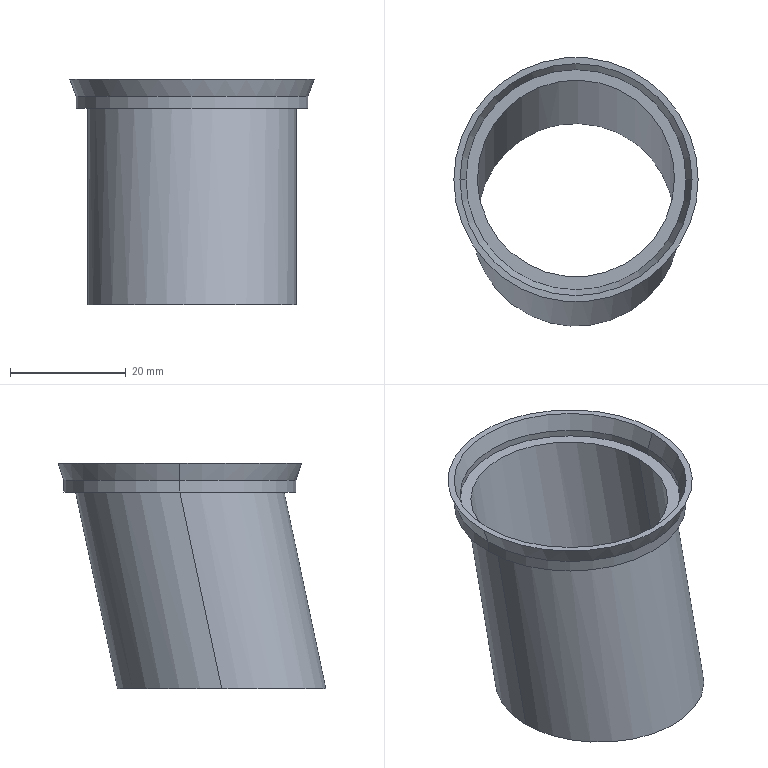Part | SolidWorks | features Extrusion 1, ICE 1, Shell 1, Sweep 1 | 1 solid | 16 faces | box 42.184 x 46.319 x 39 mm | volume 4653 mm3 | cone 4 | cylinder 4 | spline 4 | plane 4 | commonest cylinder face diameters 38 x2 40 x2
STEP:
#1=CARTESIAN_POINT('',(-19.,0.,0.1763));
#2=VERTEX_POINT('',#1);
#3=CARTESIAN_POINT('',(19.,0.,0.1763));
#4=VERTEX_POINT('',#3);
#5=CARTESIAN_POINT('',(0.,0.,0.1763));
#6=DIRECTION('',(0.,0.,1.));
#7=DIRECTION('',(1.,0.,0.));
#8=AXIS2_PLACEMENT_3D('',#5,#6,#7);
#9=CIRCLE('',#8,19.);
#10=EDGE_CURVE('',#2,#4,#9,.T.);
#11=ORIENTED_EDGE('',*,*,#10,.F.);
#12=CARTESIAN_POINT('',(-20.028,0.,3.));
#13=VERTEX_POINT('',#12);
#14=CARTESIAN_POINT('',(-19.06,0.,0.342));
#15=DIRECTION('',(-0.342,0.,0.9397));
#16=VECTOR('',#15,1000.);
#17=LINE('',#14,#16);
#18=EDGE_CURVE('',#2,#13,#17,.T.);
#19=ORIENTED_EDGE('',*,*,#18,.T.);
#20=CARTESIAN_POINT('',(20.028,0.,3.));
#21=VERTEX_POINT('',#20);
#22=CARTESIAN_POINT('',(0.,0.,3.));
#23=DIRECTION('',(0.,0.,1.));
#24=DIRECTION('',(1.,0.,0.));
#25=AXIS2_PLACEMENT_3D('',#22,#23,#24);
#26=CIRCLE('',#25,20.028);
#27=EDGE_CURVE('',#13,#21,#26,.T.);
#28=ORIENTED_EDGE('',*,*,#27,.T.);
#29=CARTESIAN_POINT('',(19.06,0.,0.342));
#30=DIRECTION('',(0.342,0.,0.9397));
#31=VECTOR('',#30,1000.);
#32=LINE('',#29,#31);
#33=EDGE_CURVE('',#4,#21,#32,.T.);
#34=ORIENTED_EDGE('',*,*,#33,.F.);
#35=EDGE_LOOP('',(#11,#19,#28,#34));
#36=FACE_OUTER_BOUND('',#35,.T.);
#37=CARTESIAN_POINT('',(0.,0.,0.342));
#38=DIRECTION('',(0.,0.,1.));
#39=DIRECTION('',(1.,0.,0.));
#40=AXIS2_PLACEMENT_3D('',#37,#38,#39);
#41=CONICAL_SURFACE('',#40,19.06,0.3491);
#42=ADVANCED_FACE('',(#36),#41,.F.);
#43=CARTESIAN_POINT('',(-19.,0.,-1.));
#44=VERTEX_POINT('',#43);
#45=CARTESIAN_POINT('',(19.,0.,-1.));
#46=VERTEX_POINT('',#45);
#47=CARTESIAN_POINT('',(0.,0.,-1.));
#48=DIRECTION('',(0.,0.,1.));
#49=DIRECTION('',(1.,0.,0.));
#50=AXIS2_PLACEMENT_3D('',#47,#48,#49);
#51=CIRCLE('',#50,19.);
#52=EDGE_CURVE('',#44,#46,#51,.T.);
#53=ORIENTED_EDGE('',*,*,#52,.F.);
#54=CARTESIAN_POINT('',(-19.,0.,-2.));
#55=DIRECTION('',(0.,0.,1.));
#56=VECTOR('',#55,1000.);
#57=LINE('',#54,#56);
#58=EDGE_CURVE('',#44,#2,#57,.T.);
#59=ORIENTED_EDGE('',*,*,#58,.T.);
#60=ORIENTED_EDGE('',*,*,#10,.T.);
#61=CARTESIAN_POINT('',(19.,0.,-2.));
#62=DIRECTION('',(0.,0.,1.));
#63=VECTOR('',#62,1000.);
#64=LINE('',#61,#63);
#65=EDGE_CURVE('',#46,#4,#64,.T.);
#66=ORIENTED_EDGE('',*,*,#65,.F.);
#67=EDGE_LOOP('',(#53,#59,#60,#66));
#68=FACE_OUTER_BOUND('',#67,.T.);
#69=CARTESIAN_POINT('',(0.,0.,-2.));
#70=DIRECTION('',(0.,0.,1.));
#71=DIRECTION('',(1.,0.,0.));
#72=AXIS2_PLACEMENT_3D('',#69,#70,#71);
#73=CYLINDRICAL_SURFACE('',#72,19.);
#74=ADVANCED_FACE('',(#68),#73,.F.);
#75=CARTESIAN_POINT('',(-17.,-7.227,-36.));
#76=VERTEX_POINT('',#75);
#77=CARTESIAN_POINT('',(17.,-7.227,-36.));
#78=VERTEX_POINT('',#77);
#79=CARTESIAN_POINT('',(-17.,-7.227,-36.));
#80=CARTESIAN_POINT('',(-17.,-6.117,-36.));
#81=CARTESIAN_POINT('',(-16.892,-5.016,-36.));
#82=CARTESIAN_POINT('',(-16.567,-3.377,-36.));
#83=CARTESIAN_POINT('',(-16.43,-2.83,-36.));
#84=CARTESIAN_POINT('',(-16.105,-1.764,-36.));
#85=CARTESIAN_POINT('',(-15.918,-1.242,-36.));
#86=CARTESIAN_POINT('',(-15.282,0.2919,-36.));
#87=CARTESIAN_POINT('',(-14.76,1.271,-36.));
#88=CARTESIAN_POINT('',(-13.512,3.136,-36.));
#89=CARTESIAN_POINT('',(-12.807,3.992,-36.));
#90=CARTESIAN_POINT('',(-11.633,5.166,-36.));
#91=CARTESIAN_POINT('',(-11.222,5.539,-36.));
#92=CARTESIAN_POINT('',(-10.359,6.246,-36.));
#93=CARTESIAN_POINT('',(-9.906,6.581,-36.));
#94=CARTESIAN_POINT('',(-8.518,7.508,-36.));
#95=CARTESIAN_POINT('',(-7.541,8.029,-36.));
#96=CARTESIAN_POINT('',(-6.003,8.667,-36.));
#97=CARTESIAN_POINT('',(-5.475,8.856,-36.));
#98=CARTESIAN_POINT('',(-4.404,9.181,-36.));
#99=CARTESIAN_POINT('',(-3.864,9.316,-36.));
#100=CARTESIAN_POINT('',(-2.234,9.64,-36.));
#101=CARTESIAN_POINT('',(-1.132,9.75,-36.));
#102=CARTESIAN_POINT('',(0.544,9.751,-36.));
#103=CARTESIAN_POINT('',(1.106,9.724,-36.));
#104=CARTESIAN_POINT('',(2.212,9.616,-36.));
#105=CARTESIAN_POINT('',(3.308,9.454,-36.));
#106=CARTESIAN_POINT('',(4.383,9.186,-36.));
#107=CARTESIAN_POINT('',(5.447,8.865,-36.));
#108=CARTESIAN_POINT('',(5.977,8.677,-36.));
#109=CARTESIAN_POINT('',(7.526,8.037,-36.));
#110=CARTESIAN_POINT('',(8.503,7.516,-36.));
#111=CARTESIAN_POINT('',(9.887,6.595,-36.));
#112=CARTESIAN_POINT('',(10.334,6.265,-36.));
#113=CARTESIAN_POINT('',(11.201,5.557,-36.));
#114=CARTESIAN_POINT('',(11.617,5.181,-36.));
#115=CARTESIAN_POINT('',(12.796,4.005,-36.));
#116=CARTESIAN_POINT('',(13.5,3.151,-36.));
#117=CARTESIAN_POINT('',(14.431,1.765,-36.));
#118=CARTESIAN_POINT('',(14.721,1.283,-36.));
#119=CARTESIAN_POINT('',(15.249,0.2992,-36.));
#120=CARTESIAN_POINT('',(15.486,-0.2022,-36.));
#121=CARTESIAN_POINT('',(16.124,-1.735,-36.));
#122=CARTESIAN_POINT('',(16.449,-2.795,-36.));
#123=CARTESIAN_POINT('',(16.89,-4.994,-36.));
#124=CARTESIAN_POINT('',(17.,-6.107,-36.));
#125=CARTESIAN_POINT('',(17.,-7.227,-36.));
#126=B_SPLINE_CURVE_WITH_KNOTS('',3,(#79,#80,#81,#82,#83,#84,#85,#86,#87,#88,#89,#90,#91,#92,#93,#94,#95,#96,#97,#98,#99,#100,#101,#102,#103,#104,#105,#106,#107,#108,#109,#110,#111,#112,#113,#114,#115,#116,#117,#118,#119,#120,#121,#122,#123,#124,#125),.UNSPECIFIED.,.F.,.F.,(4,2,2,2,2,2,2,2,2,2,2,2,2,1,2,2,2,2,2,2,2,2,2,4),(0.05282,0.05614,0.0578,0.05946,0.06278,0.0661,0.06776,0.06941,0.07273,0.07439,0.07605,0.07937,0.08103,0.08269,0.08435,0.08601,0.08933,0.09099,0.09265,0.09597,0.09763,0.09929,0.1026,0.1059),.UNSPECIFIED.);
#127=EDGE_CURVE('',#76,#78,#126,.T.);
#128=ORIENTED_EDGE('',*,*,#127,.T.);
#129=CARTESIAN_POINT('',(17.,0.2126,-1.));
#130=VERTEX_POINT('',#129);
#131=CARTESIAN_POINT('',(17.,-9.356,-46.017));
#132=DIRECTION('',(0.,0.2079,0.9781));
#133=VECTOR('',#132,1000.);
#134=LINE('',#131,#133);
#135=EDGE_CURVE('',#78,#130,#134,.T.);
#136=ORIENTED_EDGE('',*,*,#135,.T.);
#137=CARTESIAN_POINT('',(-17.,0.2126,-1.));
#138=VERTEX_POINT('',#137);
#139=CARTESIAN_POINT('',(-17.,0.2126,-1.));
#140=CARTESIAN_POINT('',(-17.,1.322,-1.));
#141=CARTESIAN_POINT('',(-16.892,2.423,-1.));
#142=CARTESIAN_POINT('',(-16.566,4.063,-1.));
#143=CARTESIAN_POINT('',(-16.429,4.61,-1.));
#144=CARTESIAN_POINT('',(-16.105,5.676,-1.));
#145=CARTESIAN_POINT('',(-15.918,6.198,-1.));
#146=CARTESIAN_POINT('',(-15.494,7.22,-1.));
#147=CARTESIAN_POINT('',(-15.258,7.72,-1.));
#148=CARTESIAN_POINT('',(-14.734,8.699,-1.));
#149=CARTESIAN_POINT('',(-14.447,9.178,-1.));
#150=CARTESIAN_POINT('',(-13.512,10.576,-1.));
#151=CARTESIAN_POINT('',(-12.808,11.431,-1.));
#152=CARTESIAN_POINT('',(-11.633,12.605,-1.));
#153=CARTESIAN_POINT('',(-11.222,12.978,-1.));
#154=CARTESIAN_POINT('',(-10.358,13.686,-1.));
#155=CARTESIAN_POINT('',(-9.906,14.021,-1.));
#156=CARTESIAN_POINT('',(-8.518,14.947,-1.));
#157=CARTESIAN_POINT('',(-7.542,15.468,-1.));
#158=CARTESIAN_POINT('',(-6.003,16.106,-1.));
#159=CARTESIAN_POINT('',(-5.474,16.296,-1.));
#160=CARTESIAN_POINT('',(-4.404,16.62,-1.));
#161=CARTESIAN_POINT('',(-3.865,16.755,-1.));
#162=CARTESIAN_POINT('',(-2.235,17.079,-1.));
#163=CARTESIAN_POINT('',(-1.133,17.189,-1.));
#164=CARTESIAN_POINT('',(0.5447,17.191,-1.));
#165=CARTESIAN_POINT('',(1.106,17.163,-1.));
#166=CARTESIAN_POINT('',(2.211,17.055,-1.));
#167=CARTESIAN_POINT('',(3.307,16.893,-1.));
#168=CARTESIAN_POINT('',(4.382,16.626,-1.));
#169=CARTESIAN_POINT('',(5.447,16.305,-1.));
#170=CARTESIAN_POINT('',(5.977,16.116,-1.));
#171=CARTESIAN_POINT('',(7.525,15.477,-1.));
#172=CARTESIAN_POINT('',(8.502,14.956,-1.));
#173=CARTESIAN_POINT('',(9.886,14.035,-1.));
#174=CARTESIAN_POINT('',(10.334,13.705,-1.));
#175=CARTESIAN_POINT('',(11.201,12.996,-1.));
#176=CARTESIAN_POINT('',(11.616,12.621,-1.));
#177=CARTESIAN_POINT('',(12.796,11.445,-1.));
#178=CARTESIAN_POINT('',(13.499,10.591,-1.));
#179=CARTESIAN_POINT('',(14.431,9.205,-1.));
#180=CARTESIAN_POINT('',(14.721,8.722,-1.));
#181=CARTESIAN_POINT('',(15.248,7.739,-1.));
#182=CARTESIAN_POINT('',(15.486,7.238,-1.));
#183=CARTESIAN_POINT('',(16.124,5.705,-1.));
#184=CARTESIAN_POINT('',(16.449,4.645,-1.));
#185=CARTESIAN_POINT('',(16.89,2.444,-1.));
#186=CARTESIAN_POINT('',(17.,1.334,-1.));
#187=CARTESIAN_POINT('',(17.,0.2126,-1.));
#188=B_SPLINE_CURVE_WITH_KNOTS('',3,(#139,#140,#141,#142,#143,#144,#145,#146,#147,#148,#149,#150,#151,#152,#153,#154,#155,#156,#157,#158,#159,#160,#161,#162,#163,#164,#165,#166,#167,#168,#169,#170,#171,#172,#173,#174,#175,#176,#177,#178,#179,#180,#181,#182,#183,#184,#185,#186,#187),.UNSPECIFIED.,.F.,.F.,(4,2,2,2,2,2,2,2,2,2,2,2,2,2,1,2,2,2,2,2,2,2,2,2,4),(0.05292,0.05623,0.05789,0.05955,0.06121,0.06287,0.06619,0.06785,0.06951,0.07283,0.07449,0.07615,0.07947,0.08113,0.08279,0.08445,0.08611,0.08943,0.09108,0.09274,0.09606,0.09772,0.09938,0.1027,0.106),.UNSPECIFIED.);
#189=EDGE_CURVE('',#138,#130,#188,.T.);
#190=ORIENTED_EDGE('',*,*,#189,.F.);
#191=CARTESIAN_POINT('',(-17.,-9.356,-46.017));
#192=DIRECTION('',(0.,0.2079,0.9781));
#193=VECTOR('',#192,1000.);
#194=LINE('',#191,#193);
#195=EDGE_CURVE('',#76,#138,#194,.T.);
#196=ORIENTED_EDGE('',*,*,#195,.F.);
#197=EDGE_LOOP('',(#128,#136,#190,#196));
#198=FACE_OUTER_BOUND('',#197,.T.);
#199=CARTESIAN_POINT('',(-17.,-7.316,-36.42));
#200=CARTESIAN_POINT('',(-17.,0.2575,-0.7887));
#201=CARTESIAN_POINT('',(-17.,-6.203,-36.406));
#202=CARTESIAN_POINT('',(-17.,1.37,-0.7748));
#203=CARTESIAN_POINT('',(-16.891,-5.091,-36.392));
#204=CARTESIAN_POINT('',(-16.891,2.483,-0.7609));
#205=CARTESIAN_POINT('',(-16.458,-2.908,-36.365));
#206=CARTESIAN_POINT('',(-16.458,4.666,-0.7337));
#207=CARTESIAN_POINT('',(-16.134,-1.838,-36.351));
#208=CARTESIAN_POINT('',(-16.134,5.736,-0.7204));
#209=CARTESIAN_POINT('',(-15.284,0.2193,-36.326));
#210=CARTESIAN_POINT('',(-15.284,7.793,-0.6949));
#211=CARTESIAN_POINT('',(-14.758,1.206,-36.314));
#212=CARTESIAN_POINT('',(-14.758,8.78,-0.6828));
#213=CARTESIAN_POINT('',(-13.523,3.059,-36.291));
#214=CARTESIAN_POINT('',(-13.523,10.632,-0.6601));
#215=CARTESIAN_POINT('',(-12.815,3.924,-36.281));
#216=CARTESIAN_POINT('',(-12.815,11.498,-0.6496));
#217=CARTESIAN_POINT('',(-11.242,5.501,-36.262));
#218=CARTESIAN_POINT('',(-11.242,13.074,-0.6306));
#219=CARTESIAN_POINT('',(-10.378,6.212,-36.253));
#220=CARTESIAN_POINT('',(-10.378,13.785,-0.6221));
#221=CARTESIAN_POINT('',(-8.528,7.451,-36.238));
#222=CARTESIAN_POINT('',(-8.528,15.025,-0.6073));
#223=CARTESIAN_POINT('',(-7.541,7.98,-36.232));
#224=CARTESIAN_POINT('',(-7.541,15.554,-0.6011));
#225=CARTESIAN_POINT('',(-5.484,8.834,-36.222));
#226=CARTESIAN_POINT('',(-5.484,16.408,-0.591));
#227=CARTESIAN_POINT('',(-4.413,9.16,-36.218));
#228=CARTESIAN_POINT('',(-4.413,16.734,-0.5872));
#229=CARTESIAN_POINT('',(-2.228,9.596,-36.213));
#230=CARTESIAN_POINT('',(-2.228,17.169,-0.5821));
#231=CARTESIAN_POINT('',(-1.114,9.706,-36.212));
#232=CARTESIAN_POINT('',(-1.114,17.279,-0.5808));
#233=CARTESIAN_POINT('',(1.114,9.706,-36.212));
#234=CARTESIAN_POINT('',(1.114,17.279,-0.5808));
#235=CARTESIAN_POINT('',(2.228,9.596,-36.213));
#236=CARTESIAN_POINT('',(2.228,17.169,-0.5821));
#237=CARTESIAN_POINT('',(4.413,9.16,-36.218));
#238=CARTESIAN_POINT('',(4.413,16.734,-0.5872));
#239=CARTESIAN_POINT('',(5.484,8.834,-36.222));
#240=CARTESIAN_POINT('',(5.484,16.408,-0.591));
#241=CARTESIAN_POINT('',(7.541,7.98,-36.232));
#242=CARTESIAN_POINT('',(7.541,15.554,-0.6011));
#243=CARTESIAN_POINT('',(8.528,7.451,-36.238));
#244=CARTESIAN_POINT('',(8.528,15.025,-0.6073));
#245=CARTESIAN_POINT('',(10.378,6.212,-36.253));
#246=CARTESIAN_POINT('',(10.378,13.785,-0.6221));
#247=CARTESIAN_POINT('',(11.242,5.501,-36.262));
#248=CARTESIAN_POINT('',(11.242,13.074,-0.6306));
#249=CARTESIAN_POINT('',(12.815,3.924,-36.281));
#250=CARTESIAN_POINT('',(12.815,11.498,-0.6496));
#251=CARTESIAN_POINT('',(13.523,3.059,-36.291));
#252=CARTESIAN_POINT('',(13.523,10.632,-0.6601));
#253=CARTESIAN_POINT('',(14.758,1.206,-36.314));
#254=CARTESIAN_POINT('',(14.758,8.78,-0.6828));
#255=CARTESIAN_POINT('',(15.284,0.2193,-36.326));
#256=CARTESIAN_POINT('',(15.284,7.793,-0.6949));
#257=CARTESIAN_POINT('',(16.134,-1.838,-36.351));
#258=CARTESIAN_POINT('',(16.134,5.736,-0.7204));
#259=CARTESIAN_POINT('',(16.458,-2.908,-36.365));
#260=CARTESIAN_POINT('',(16.458,4.666,-0.7337));
#261=CARTESIAN_POINT('',(16.891,-5.091,-36.392));
#262=CARTESIAN_POINT('',(16.891,2.483,-0.7609));
#263=CARTESIAN_POINT('',(17.,-6.203,-36.406));
#264=CARTESIAN_POINT('',(17.,1.37,-0.7748));
#265=CARTESIAN_POINT('',(17.,-7.316,-36.42));
#266=CARTESIAN_POINT('',(17.,0.2575,-0.7887));
#267=B_SPLINE_SURFACE_WITH_KNOTS('',3,1,((#199,#200),(#201,#202),(#203,#204),(#205,#206),(#207,#208),(#209,#210),(#211,#212),(#213,#214),(#215,#216),(#217,#218),(#219,#220),(#221,#222),(#223,#224),(#225,#226),(#227,#228),(#229,#230),(#231,#232),(#233,#234),(#235,#236),(#237,#238),(#239,#240),(#241,#242),(#243,#244),(#245,#246),(#247,#248),(#249,#250),(#251,#252),(#253,#254),(#255,#256),(#257,#258),(#259,#260),(#261,#262),(#263,#264),(#265,#266)),.UNSPECIFIED.,.F.,.F.,.F.,(4,2,2,2,2,2,2,2,2,2,2,2,2,2,2,2,4),(2,2),(0.,0.0625,0.125,0.1875,0.25,0.3125,0.375,0.4375,0.5,0.5625,0.625,0.6875,0.75,0.8125,0.875,0.9375,1.),(0.,1.),.UNSPECIFIED.);
#268=ADVANCED_FACE('',(#198),#267,.T.);
#269=CARTESIAN_POINT('',(20.,0.,0.));
#270=VERTEX_POINT('',#269);
#271=CARTESIAN_POINT('',(-20.,0.,0.));
#272=VERTEX_POINT('',#271);
#273=CARTESIAN_POINT('',(0.,0.,0.));
#274=DIRECTION('',(0.,0.,1.));
#275=DIRECTION('',(1.,0.,0.));
#276=AXIS2_PLACEMENT_3D('',#273,#274,#275);
#277=CIRCLE('',#276,20.);
#278=EDGE_CURVE('',#270,#272,#277,.T.);
#279=ORIENTED_EDGE('',*,*,#278,.T.);
#280=CARTESIAN_POINT('',(-21.092,0.,3.));
#281=VERTEX_POINT('',#280);
#282=CARTESIAN_POINT('',(-20.,0.,0.));
#283=DIRECTION('',(-0.342,0.,0.9397));
#284=VECTOR('',#283,1000.);
#285=LINE('',#282,#284);
#286=EDGE_CURVE('',#272,#281,#285,.T.);
#287=ORIENTED_EDGE('',*,*,#286,.T.);
#288=CARTESIAN_POINT('',(21.092,0.,3.));
#289=VERTEX_POINT('',#288);
#290=CARTESIAN_POINT('',(0.,0.,3.));
#291=DIRECTION('',(0.,0.,1.));
#292=DIRECTION('',(1.,0.,0.));
#293=AXIS2_PLACEMENT_3D('',#290,#291,#292);
#294=CIRCLE('',#293,21.092);
#295=EDGE_CURVE('',#289,#281,#294,.T.);
#296=ORIENTED_EDGE('',*,*,#295,.F.);
#297=CARTESIAN_POINT('',(20.,0.,0.));
#298=DIRECTION('',(0.342,0.,0.9397));
#299=VECTOR('',#298,1000.);
#300=LINE('',#297,#299);
#301=EDGE_CURVE('',#270,#289,#300,.T.);
#302=ORIENTED_EDGE('',*,*,#301,.F.);
#303=EDGE_LOOP('',(#279,#287,#296,#302));
#304=FACE_OUTER_BOUND('',#303,.T.);
#305=CARTESIAN_POINT('',(0.,0.,0.));
#306=DIRECTION('',(0.,0.,1.));
#307=DIRECTION('',(1.,0.,0.));
#308=AXIS2_PLACEMENT_3D('',#305,#306,#307);
#309=CONICAL_SURFACE('',#308,20.,0.3491);
#310=ADVANCED_FACE('',(#304),#309,.T.);
#311=CARTESIAN_POINT('',(20.,0.,-2.));
#312=VERTEX_POINT('',#311);
#313=CARTESIAN_POINT('',(-20.,0.,-2.));
#314=VERTEX_POINT('',#313);
#315=CARTESIAN_POINT('',(0.,0.,-2.));
#316=DIRECTION('',(0.,0.,1.));
#317=DIRECTION('',(1.,0.,0.));
#318=AXIS2_PLACEMENT_3D('',#315,#316,#317);
#319=CIRCLE('',#318,20.);
#320=EDGE_CURVE('',#312,#314,#319,.T.);
#321=ORIENTED_EDGE('',*,*,#320,.T.);
#322=CARTESIAN_POINT('',(-20.,0.,-2.));
#323=DIRECTION('',(0.,0.,1.));
#324=VECTOR('',#323,1000.);
#325=LINE('',#322,#324);
#326=EDGE_CURVE('',#314,#272,#325,.T.);
#327=ORIENTED_EDGE('',*,*,#326,.T.);
#328=ORIENTED_EDGE('',*,*,#278,.F.);
#329=CARTESIAN_POINT('',(20.,0.,-2.));
#330=DIRECTION('',(0.,0.,1.));
#331=VECTOR('',#330,1000.);
#332=LINE('',#329,#331);
#333=EDGE_CURVE('',#312,#270,#332,.T.);
#334=ORIENTED_EDGE('',*,*,#333,.F.);
#335=EDGE_LOOP('',(#321,#327,#328,#334));
#336=FACE_OUTER_BOUND('',#335,.T.);
#337=CARTESIAN_POINT('',(0.,0.,-2.));
#338=DIRECTION('',(0.,0.,1.));
#339=DIRECTION('',(1.,0.,0.));
#340=AXIS2_PLACEMENT_3D('',#337,#338,#339);
#341=CYLINDRICAL_SURFACE('',#340,20.);
#342=ADVANCED_FACE('',(#336),#341,.T.);
#343=CARTESIAN_POINT('',(18.,-7.227,-36.));
#344=VERTEX_POINT('',#343);
#345=CARTESIAN_POINT('',(-18.,-7.227,-36.));
#346=VERTEX_POINT('',#345);
#347=CARTESIAN_POINT('',(18.,-7.227,-36.));
#348=CARTESIAN_POINT('',(18.,-8.406,-36.));
#349=CARTESIAN_POINT('',(17.884,-9.582,-36.));
#350=CARTESIAN_POINT('',(17.539,-11.317,-36.));
#351=CARTESIAN_POINT('',(17.396,-11.888,-36.));
#352=CARTESIAN_POINT('',(17.054,-13.015,-36.));
#353=CARTESIAN_POINT('',(16.855,-13.572,-36.));
#354=CARTESIAN_POINT('',(16.404,-14.659,-36.));
#355=CARTESIAN_POINT('',(16.153,-15.191,-36.));
#356=CARTESIAN_POINT('',(15.597,-16.231,-36.));
#357=CARTESIAN_POINT('',(15.294,-16.738,-36.));
#358=CARTESIAN_POINT('',(14.313,-18.205,-36.));
#359=CARTESIAN_POINT('',(13.561,-19.122,-36.));
#360=CARTESIAN_POINT('',(12.313,-20.37,-36.));
#361=CARTESIAN_POINT('',(11.875,-20.767,-36.));
#362=CARTESIAN_POINT('',(10.964,-21.514,-36.));
#363=CARTESIAN_POINT('',(10.492,-21.865,-36.));
#364=CARTESIAN_POINT('',(9.512,-22.519,-36.));
#365=CARTESIAN_POINT('',(9.005,-22.823,-36.));
#366=CARTESIAN_POINT('',(7.968,-23.378,-36.));
#367=CARTESIAN_POINT('',(7.436,-23.63,-36.));
#368=CARTESIAN_POINT('',(6.345,-24.082,-36.));
#369=CARTESIAN_POINT('',(5.79,-24.28,-36.));
#370=CARTESIAN_POINT('',(4.665,-24.622,-36.));
#371=CARTESIAN_POINT('',(4.091,-24.766,-36.));
#372=CARTESIAN_POINT('',(2.936,-24.996,-36.));
#373=CARTESIAN_POINT('',(2.354,-25.082,-36.));
#374=CARTESIAN_POINT('',(1.182,-25.198,-36.));
#375=CARTESIAN_POINT('',(0.5909,-25.227,-36.));
#376=CARTESIAN_POINT('',(-1.175,-25.227,-36.));
#377=CARTESIAN_POINT('',(-2.354,-25.111,-36.));
#378=CARTESIAN_POINT('',(-4.085,-24.767,-36.));
#379=CARTESIAN_POINT('',(-4.658,-24.624,-36.));
#380=CARTESIAN_POINT('',(-5.786,-24.282,-36.));
#381=CARTESIAN_POINT('',(-6.34,-24.084,-36.));
#382=CARTESIAN_POINT('',(-7.428,-23.633,-36.));
#383=CARTESIAN_POINT('',(-7.963,-23.38,-36.));
#384=CARTESIAN_POINT('',(-9.001,-22.826,-36.));
#385=CARTESIAN_POINT('',(-9.506,-22.523,-36.));
#386=CARTESIAN_POINT('',(-10.977,-21.541,-36.));
#387=CARTESIAN_POINT('',(-11.891,-20.792,-36.));
#388=CARTESIAN_POINT('',(-13.142,-19.541,-36.));
#389=CARTESIAN_POINT('',(-13.537,-19.105,-36.));
#390=CARTESIAN_POINT('',(-14.284,-18.195,-36.));
#391=CARTESIAN_POINT('',(-14.637,-17.72,-36.));
#392=CARTESIAN_POINT('',(-15.291,-16.741,-36.));
#393=CARTESIAN_POINT('',(-15.594,-16.237,-36.));
#394=CARTESIAN_POINT('',(-16.15,-15.198,-36.));
#395=CARTESIAN_POINT('',(-16.403,-14.664,-36.));
#396=CARTESIAN_POINT('',(-17.078,-13.033,-36.));
#397=CARTESIAN_POINT('',(-17.423,-11.899,-36.));
#398=CARTESIAN_POINT('',(-17.883,-9.589,-36.));
#399=CARTESIAN_POINT('',(-18.,-8.408,-36.));
#400=CARTESIAN_POINT('',(-18.,-7.227,-36.));
#401=B_SPLINE_CURVE_WITH_KNOTS('',3,(#347,#348,#349,#350,#351,#352,#353,#354,#355,#356,#357,#358,#359,#360,#361,#362,#363,#364,#365,#366,#367,#368,#369,#370,#371,#372,#373,#374,#375,#376,#377,#378,#379,#380,#381,#382,#383,#384,#385,#386,#387,#388,#389,#390,#391,#392,#393,#394,#395,#396,#397,#398,#399,#400),.UNSPECIFIED.,.F.,.F.,(4,2,2,2,2,2,2,2,2,2,2,2,2,2,2,2,2,2,2,2,2,2,2,2,2,2,4),(0.05648,0.06001,0.06178,0.06354,0.06531,0.06707,0.0706,0.07237,0.07413,0.0759,0.07766,0.07943,0.08119,0.08296,0.08472,0.08825,0.09002,0.09178,0.09355,0.09531,0.09884,0.1006,0.1024,0.1041,0.1059,0.1094,0.113),.UNSPECIFIED.);
#402=EDGE_CURVE('',#344,#346,#401,.T.);
#403=ORIENTED_EDGE('',*,*,#402,.F.);
#404=CARTESIAN_POINT('',(18.,0.,-2.));
#405=VERTEX_POINT('',#404);
#406=CARTESIAN_POINT('',(18.,-9.356,-46.017));
#407=DIRECTION('',(0.,0.2079,0.9781));
#408=VECTOR('',#407,1000.);
#409=LINE('',#406,#408);
#410=EDGE_CURVE('',#344,#405,#409,.T.);
#411=ORIENTED_EDGE('',*,*,#410,.T.);
#412=CARTESIAN_POINT('',(-18.,0.,-2.));
#413=VERTEX_POINT('',#412);
#414=CARTESIAN_POINT('',(0.,0.,-2.));
#415=DIRECTION('',(0.,0.,-1.));
#416=DIRECTION('',(-1.,0.,0.));
#417=AXIS2_PLACEMENT_3D('',#414,#415,#416);
#418=CIRCLE('',#417,18.);
#419=EDGE_CURVE('',#405,#413,#418,.T.);
#420=ORIENTED_EDGE('',*,*,#419,.T.);
#421=CARTESIAN_POINT('',(-18.,-9.356,-46.017));
#422=DIRECTION('',(0.,0.2079,0.9781));
#423=VECTOR('',#422,1000.);
#424=LINE('',#421,#423);
#425=EDGE_CURVE('',#346,#413,#424,.T.);
#426=ORIENTED_EDGE('',*,*,#425,.F.);
#427=EDGE_LOOP('',(#403,#411,#420,#426));
#428=FACE_OUTER_BOUND('',#427,.T.);
#429=CARTESIAN_POINT('',(18.,-7.227,-36.));
#430=CARTESIAN_POINT('',(18.,0.,-2.));
#431=CARTESIAN_POINT('',(18.,-43.227,-36.));
#432=CARTESIAN_POINT('',(18.,-36.,-2.));
#433=CARTESIAN_POINT('',(-18.,-43.227,-36.));
#434=CARTESIAN_POINT('',(-18.,-36.,-2.));
#435=CARTESIAN_POINT('',(-18.,-7.227,-36.));
#436=CARTESIAN_POINT('',(-18.,0.,-2.));
#437=(BOUNDED_SURFACE()B_SPLINE_SURFACE(3,1,((#429,#430),(#431,#432),(#433,#434),(#435,#436)),.UNSPECIFIED.,.F.,.F.,.F.)B_SPLINE_SURFACE_WITH_KNOTS((4,4),(2,2),(0.,1.),(0.,1.),.UNSPECIFIED.)GEOMETRIC_REPRESENTATION_ITEM()RATIONAL_B_SPLINE_SURFACE(((1.,1.),(0.3333,0.3333),(0.3333,0.3333),(1.,1.)))REPRESENTATION_ITEM('')SURFACE());
#438=ADVANCED_FACE('',(#428),#437,.F.);
#439=ORIENTED_EDGE('',*,*,#410,.F.);
#440=CARTESIAN_POINT('',(-18.,-7.227,-36.));
#441=CARTESIAN_POINT('',(-18.,-6.637,-36.));
#442=CARTESIAN_POINT('',(-17.971,-6.049,-36.));
#443=CARTESIAN_POINT('',(-17.856,-4.877,-36.));
#444=CARTESIAN_POINT('',(-17.769,-4.293,-36.));
#445=CARTESIAN_POINT('',(-17.539,-3.137,-36.));
#446=CARTESIAN_POINT('',(-17.396,-2.566,-36.));
#447=CARTESIAN_POINT('',(-17.054,-1.439,-36.));
#448=CARTESIAN_POINT('',(-16.855,-0.8819,-36.));
#449=CARTESIAN_POINT('',(-16.179,0.7493,-36.));
#450=CARTESIAN_POINT('',(-15.62,1.795,-36.));
#451=CARTESIAN_POINT('',(-14.64,3.263,-36.));
#452=CARTESIAN_POINT('',(-14.288,3.737,-36.));
#453=CARTESIAN_POINT('',(-13.54,4.648,-36.));
#454=CARTESIAN_POINT('',(-13.145,5.084,-36.));
#455=CARTESIAN_POINT('',(-12.312,5.917,-36.));
#456=CARTESIAN_POINT('',(-11.874,6.314,-36.));
#457=CARTESIAN_POINT('',(-10.963,7.061,-36.));
#458=CARTESIAN_POINT('',(-10.491,7.412,-36.));
#459=CARTESIAN_POINT('',(-9.02,8.395,-36.));
#460=CARTESIAN_POINT('',(-7.977,8.952,-36.));
#461=CARTESIAN_POINT('',(-6.343,9.629,-36.));
#462=CARTESIAN_POINT('',(-5.789,9.827,-36.));
#463=CARTESIAN_POINT('',(-4.662,10.169,-36.));
#464=CARTESIAN_POINT('',(-4.088,10.313,-36.));
#465=CARTESIAN_POINT('',(-2.933,10.542,-36.));
#466=CARTESIAN_POINT('',(-2.351,10.629,-36.));
#467=CARTESIAN_POINT('',(-1.178,10.744,-36.));
#468=CARTESIAN_POINT('',(-0.588,10.773,-36.));
#469=CARTESIAN_POINT('',(1.177,10.773,-36.));
#470=CARTESIAN_POINT('',(2.357,10.657,-36.));
#471=CARTESIAN_POINT('',(4.089,10.312,-36.));
#472=CARTESIAN_POINT('',(4.662,10.169,-36.));
#473=CARTESIAN_POINT('',(5.79,9.827,-36.));
#474=CARTESIAN_POINT('',(6.344,9.628,-36.));
#475=CARTESIAN_POINT('',(7.432,9.178,-36.));
#476=CARTESIAN_POINT('',(7.967,8.925,-36.));
#477=CARTESIAN_POINT('',(9.005,8.37,-36.));
#478=CARTESIAN_POINT('',(9.51,8.067,-36.));
#479=CARTESIAN_POINT('',(10.491,7.411,-36.));
#480=CARTESIAN_POINT('',(10.964,7.061,-36.));
#481=CARTESIAN_POINT('',(11.874,6.314,-36.));
#482=CARTESIAN_POINT('',(12.312,5.917,-36.));
#483=CARTESIAN_POINT('',(13.145,5.084,-36.));
#484=CARTESIAN_POINT('',(13.54,4.648,-36.));
#485=CARTESIAN_POINT('',(14.288,3.737,-36.));
#486=CARTESIAN_POINT('',(14.64,3.262,-36.));
#487=CARTESIAN_POINT('',(15.621,1.794,-36.));
#488=CARTESIAN_POINT('',(16.18,0.7483,-36.));
#489=CARTESIAN_POINT('',(16.855,-0.8825,-36.));
#490=CARTESIAN_POINT('',(17.054,-1.439,-36.));
#491=CARTESIAN_POINT('',(17.396,-2.567,-36.));
#492=CARTESIAN_POINT('',(17.539,-3.138,-36.));
#493=CARTESIAN_POINT('',(17.769,-4.293,-36.));
#494=CARTESIAN_POINT('',(17.856,-4.878,-36.));
#495=CARTESIAN_POINT('',(17.971,-6.05,-36.));
#496=CARTESIAN_POINT('',(18.,-6.637,-36.));
#497=CARTESIAN_POINT('',(18.,-7.227,-36.));
#498=B_SPLINE_CURVE_WITH_KNOTS('',3,(#440,#441,#442,#443,#444,#445,#446,#447,#448,#449,#450,#451,#452,#453,#454,#455,#456,#457,#458,#459,#460,#461,#462,#463,#464,#465,#466,#467,#468,#469,#470,#471,#472,#473,#474,#475,#476,#477,#478,#479,#480,#481,#482,#483,#484,#485,#486,#487,#488,#489,#490,#491,#492,#493,#494,#495,#496,#497),.UNSPECIFIED.,.F.,.F.,(4,2,2,2,2,2,2,2,2,2,2,2,2,2,2,2,2,2,2,2,2,2,2,2,2,2,2,2,4),(0.,0.001765,0.00353,0.005295,0.007061,0.01059,0.01236,0.01412,0.01589,0.01765,0.02118,0.02295,0.02471,0.02648,0.02824,0.03177,0.03354,0.0353,0.03707,0.03883,0.0406,0.04236,0.04413,0.04589,0.04942,0.05119,0.05295,0.05472,0.05648),.UNSPECIFIED.);
#499=EDGE_CURVE('',#346,#344,#498,.T.);
#500=ORIENTED_EDGE('',*,*,#499,.F.);
#501=ORIENTED_EDGE('',*,*,#425,.T.);
#502=CARTESIAN_POINT('',(0.,0.,-2.));
#503=DIRECTION('',(0.,0.,-1.));
#504=DIRECTION('',(-1.,0.,0.));
#505=AXIS2_PLACEMENT_3D('',#502,#503,#504);
#506=CIRCLE('',#505,18.);
#507=EDGE_CURVE('',#413,#405,#506,.T.);
#508=ORIENTED_EDGE('',*,*,#507,.T.);
#509=EDGE_LOOP('',(#439,#500,#501,#508));
#510=FACE_OUTER_BOUND('',#509,.T.);
#511=CARTESIAN_POINT('',(-18.,-7.227,-36.));
#512=CARTESIAN_POINT('',(-18.,0.,-2.));
#513=CARTESIAN_POINT('',(-18.,28.773,-36.));
#514=CARTESIAN_POINT('',(-18.,36.,-2.));
#515=CARTESIAN_POINT('',(18.,28.773,-36.));
#516=CARTESIAN_POINT('',(18.,36.,-2.));
#517=CARTESIAN_POINT('',(18.,-7.227,-36.));
#518=CARTESIAN_POINT('',(18.,0.,-2.));
#519=(BOUNDED_SURFACE()B_SPLINE_SURFACE(3,1,((#511,#512),(#513,#514),(#515,#516),(#517,#518)),.UNSPECIFIED.,.F.,.F.,.F.)B_SPLINE_SURFACE_WITH_KNOTS((4,4),(2,2),(0.,1.),(0.,1.),.UNSPECIFIED.)GEOMETRIC_REPRESENTATION_ITEM()RATIONAL_B_SPLINE_SURFACE(((1.,1.),(0.3333,0.3333),(0.3333,0.3333),(1.,1.)))REPRESENTATION_ITEM('')SURFACE());
#520=ADVANCED_FACE('',(#510),#519,.F.);
#521=ORIENTED_EDGE('',*,*,#320,.F.);
#522=CARTESIAN_POINT('',(0.,0.,-2.));
#523=DIRECTION('',(0.,0.,1.));
#524=DIRECTION('',(1.,0.,0.));
#525=AXIS2_PLACEMENT_3D('',#522,#523,#524);
#526=CIRCLE('',#525,20.);
#527=EDGE_CURVE('',#314,#312,#526,.T.);
#528=ORIENTED_EDGE('',*,*,#527,.F.);
#529=EDGE_LOOP('',(#521,#528));
#530=FACE_OUTER_BOUND('',#529,.T.);
#531=ORIENTED_EDGE('',*,*,#507,.F.);
#532=ORIENTED_EDGE('',*,*,#419,.F.);
#533=EDGE_LOOP('',(#531,#532));
#534=FACE_BOUND('',#533,.T.);
#535=CARTESIAN_POINT('',(0.,0.,-2.));
#536=DIRECTION('',(0.,0.,1.));
#537=DIRECTION('',(1.,0.,0.));
#538=AXIS2_PLACEMENT_3D('',#535,#536,#537);
#539=PLANE('',#538);
#540=ADVANCED_FACE('',(#530,#534),#539,.F.);
#541=ORIENTED_EDGE('',*,*,#326,.F.);
#542=ORIENTED_EDGE('',*,*,#527,.T.);
#543=ORIENTED_EDGE('',*,*,#333,.T.);
#544=CARTESIAN_POINT('',(0.,0.,0.));
#545=DIRECTION('',(0.,0.,1.));
#546=DIRECTION('',(1.,0.,0.));
#547=AXIS2_PLACEMENT_3D('',#544,#545,#546);
#548=CIRCLE('',#547,20.);
#549=EDGE_CURVE('',#272,#270,#548,.T.);
#550=ORIENTED_EDGE('',*,*,#549,.F.);
#551=EDGE_LOOP('',(#541,#542,#543,#550));
#552=FACE_OUTER_BOUND('',#551,.T.);
#553=CARTESIAN_POINT('',(0.,0.,-2.));
#554=DIRECTION('',(0.,0.,1.));
#555=DIRECTION('',(1.,0.,0.));
#556=AXIS2_PLACEMENT_3D('',#553,#554,#555);
#557=CYLINDRICAL_SURFACE('',#556,20.);
#558=ADVANCED_FACE('',(#552),#557,.T.);
#559=ORIENTED_EDGE('',*,*,#286,.F.);
#560=ORIENTED_EDGE('',*,*,#549,.T.);
#561=ORIENTED_EDGE('',*,*,#301,.T.);
#562=CARTESIAN_POINT('',(0.,0.,3.));
#563=DIRECTION('',(0.,0.,1.));
#564=DIRECTION('',(1.,0.,0.));
#565=AXIS2_PLACEMENT_3D('',#562,#563,#564);
#566=CIRCLE('',#565,21.092);
#567=EDGE_CURVE('',#281,#289,#566,.T.);
#568=ORIENTED_EDGE('',*,*,#567,.F.);
#569=EDGE_LOOP('',(#559,#560,#561,#568));
#570=FACE_OUTER_BOUND('',#569,.T.);
#571=CARTESIAN_POINT('',(0.,0.,0.));
#572=DIRECTION('',(0.,0.,1.));
#573=DIRECTION('',(1.,0.,0.));
#574=AXIS2_PLACEMENT_3D('',#571,#572,#573);
#575=CONICAL_SURFACE('',#574,20.,0.3491);
#576=ADVANCED_FACE('',(#570),#575,.T.);
#577=CARTESIAN_POINT('',(0.,0.,3.));
#578=DIRECTION('',(0.,0.,1.));
#579=DIRECTION('',(1.,0.,0.));
#580=AXIS2_PLACEMENT_3D('',#577,#578,#579);
#581=CIRCLE('',#580,20.028);
#582=EDGE_CURVE('',#21,#13,#581,.T.);
#583=ORIENTED_EDGE('',*,*,#582,.F.);
#584=ORIENTED_EDGE('',*,*,#27,.F.);
#585=EDGE_LOOP('',(#583,#584));
#586=FACE_BOUND('',#585,.T.);
#587=ORIENTED_EDGE('',*,*,#295,.T.);
#588=ORIENTED_EDGE('',*,*,#567,.T.);
#589=EDGE_LOOP('',(#587,#588));
#590=FACE_OUTER_BOUND('',#589,.T.);
#591=CARTESIAN_POINT('',(0.,0.,3.));
#592=DIRECTION('',(0.,0.,1.));
#593=DIRECTION('',(1.,0.,0.));
#594=AXIS2_PLACEMENT_3D('',#591,#592,#593);
#595=PLANE('',#594);
#596=ADVANCED_FACE('',(#586,#590),#595,.T.);
#597=ORIENTED_EDGE('',*,*,#127,.F.);
#598=CARTESIAN_POINT('',(17.,-7.227,-36.));
#599=CARTESIAN_POINT('',(17.,-7.787,-36.));
#600=CARTESIAN_POINT('',(16.972,-8.347,-36.));
#601=CARTESIAN_POINT('',(16.863,-9.452,-36.));
#602=CARTESIAN_POINT('',(16.699,-10.547,-36.));
#603=CARTESIAN_POINT('',(16.43,-11.623,-36.));
#604=CARTESIAN_POINT('',(16.106,-12.688,-36.));
#605=CARTESIAN_POINT('',(15.916,-13.218,-36.));
#606=CARTESIAN_POINT('',(15.274,-14.764,-36.));
#607=CARTESIAN_POINT('',(14.751,-15.739,-36.));
#608=CARTESIAN_POINT('',(13.825,-17.122,-36.));
#609=CARTESIAN_POINT('',(13.494,-17.569,-36.));
#610=CARTESIAN_POINT('',(12.781,-18.435,-36.));
#611=CARTESIAN_POINT('',(12.406,-18.848,-36.));
#612=CARTESIAN_POINT('',(11.227,-20.023,-36.));
#613=CARTESIAN_POINT('',(10.371,-20.725,-36.));
#614=CARTESIAN_POINT('',(8.98,-21.653,-36.));
#615=CARTESIAN_POINT('',(8.497,-21.942,-36.));
#616=CARTESIAN_POINT('',(7.513,-22.467,-36.));
#617=CARTESIAN_POINT('',(7.012,-22.703,-36.));
#618=CARTESIAN_POINT('',(5.989,-23.126,-36.));
#619=CARTESIAN_POINT('',(5.468,-23.312,-36.));
#620=CARTESIAN_POINT('',(4.406,-23.634,-36.));
#621=CARTESIAN_POINT('',(3.863,-23.77,-36.));
#622=CARTESIAN_POINT('',(2.214,-24.097,-36.));
#623=CARTESIAN_POINT('',(1.111,-24.204,-36.));
#624=CARTESIAN_POINT('',(-0.55,-24.205,-36.));
#625=CARTESIAN_POINT('',(-1.105,-24.178,-36.));
#626=CARTESIAN_POINT('',(-2.216,-24.069,-36.));
#627=CARTESIAN_POINT('',(-2.773,-23.986,-36.));
#628=CARTESIAN_POINT('',(-4.409,-23.661,-36.));
#629=CARTESIAN_POINT('',(-5.468,-23.34,-36.));
#630=CARTESIAN_POINT('',(-7.009,-22.704,-36.));
#631=CARTESIAN_POINT('',(-7.517,-22.465,-36.));
#632=CARTESIAN_POINT('',(-8.504,-21.938,-36.));
#633=CARTESIAN_POINT('',(-8.981,-21.653,-36.));
#634=CARTESIAN_POINT('',(-10.363,-20.731,-36.));
#635=CARTESIAN_POINT('',(-11.221,-20.03,-36.));
#636=CARTESIAN_POINT('',(-12.408,-18.845,-36.));
#637=CARTESIAN_POINT('',(-12.786,-18.429,-36.));
#638=CARTESIAN_POINT('',(-13.492,-17.571,-36.));
#639=CARTESIAN_POINT('',(-14.152,-16.682,-36.));
#640=CARTESIAN_POINT('',(-14.723,-15.732,-36.));
#641=CARTESIAN_POINT('',(-15.249,-14.752,-36.));
#642=CARTESIAN_POINT('',(-15.49,-14.244,-36.));
#643=CARTESIAN_POINT('',(-16.132,-12.696,-36.));
#644=CARTESIAN_POINT('',(-16.454,-11.637,-36.));
#645=CARTESIAN_POINT('',(-16.78,-10.006,-36.));
#646=CARTESIAN_POINT('',(-16.862,-9.456,-36.));
#647=CARTESIAN_POINT('',(-16.973,-8.341,-36.));
#648=CARTESIAN_POINT('',(-17.,-7.782,-36.));
#649=CARTESIAN_POINT('',(-17.,-7.227,-36.));
#650=B_SPLINE_CURVE_WITH_KNOTS('',3,(#598,#599,#600,#601,#602,#603,#604,#605,#606,#607,#608,#609,#610,#611,#612,#613,#614,#615,#616,#617,#618,#619,#620,#621,#622,#623,#624,#625,#626,#627,#628,#629,#630,#631,#632,#633,#634,#635,#636,#637,#638,#639,#640,#641,#642,#643,#644,#645,#646,#647,#648,#649),.UNSPECIFIED.,.F.,.F.,(4,2,1,2,2,2,2,2,2,2,2,2,2,2,2,2,2,2,2,2,2,1,2,2,2,2,4),(0.1059,0.1076,0.1092,0.1109,0.1126,0.1159,0.1175,0.1192,0.1225,0.1242,0.1258,0.1275,0.1292,0.1325,0.1341,0.1358,0.1391,0.1408,0.1424,0.1458,0.1474,0.1491,0.1507,0.1524,0.1557,0.1574,0.159),.UNSPECIFIED.);
#651=EDGE_CURVE('',#78,#76,#650,.T.);
#652=ORIENTED_EDGE('',*,*,#651,.F.);
#653=EDGE_LOOP('',(#597,#652));
#654=FACE_BOUND('',#653,.T.);
#655=ORIENTED_EDGE('',*,*,#499,.T.);
#656=ORIENTED_EDGE('',*,*,#402,.T.);
#657=EDGE_LOOP('',(#655,#656));
#658=FACE_OUTER_BOUND('',#657,.T.);
#659=CARTESIAN_POINT('',(0.,0.,-36.));
#660=DIRECTION('',(0.,0.,-1.));
#661=DIRECTION('',(-1.,0.,0.));
#662=AXIS2_PLACEMENT_3D('',#659,#660,#661);
#663=PLANE('',#662);
#664=ADVANCED_FACE('',(#654,#658),#663,.T.);
#665=ORIENTED_EDGE('',*,*,#135,.F.);
#666=ORIENTED_EDGE('',*,*,#651,.T.);
#667=ORIENTED_EDGE('',*,*,#195,.T.);
#668=CARTESIAN_POINT('',(17.,0.2126,-1.));
#669=CARTESIAN_POINT('',(17.,-0.348,-1.));
#670=CARTESIAN_POINT('',(16.972,-0.9068,-1.));
#671=CARTESIAN_POINT('',(16.863,-2.012,-1.));
#672=CARTESIAN_POINT('',(16.781,-2.559,-1.));
#673=CARTESIAN_POINT('',(16.565,-3.644,-1.));
#674=CARTESIAN_POINT('',(16.43,-4.182,-1.));
#675=CARTESIAN_POINT('',(16.106,-5.248,-1.));
#676=CARTESIAN_POINT('',(15.916,-5.778,-1.));
#677=CARTESIAN_POINT('',(15.274,-7.323,-1.));
#678=CARTESIAN_POINT('',(14.751,-8.299,-1.));
#679=CARTESIAN_POINT('',(13.826,-9.682,-1.));
#680=CARTESIAN_POINT('',(13.493,-10.129,-1.));
#681=CARTESIAN_POINT('',(12.781,-10.996,-1.));
#682=CARTESIAN_POINT('',(12.406,-11.408,-1.));
#683=CARTESIAN_POINT('',(11.228,-12.583,-1.));
#684=CARTESIAN_POINT('',(10.372,-13.285,-1.));
#685=CARTESIAN_POINT('',(8.98,-14.214,-1.));
#686=CARTESIAN_POINT('',(8.497,-14.503,-1.));
#687=CARTESIAN_POINT('',(7.514,-15.027,-1.));
#688=CARTESIAN_POINT('',(7.013,-15.263,-1.));
#689=CARTESIAN_POINT('',(5.99,-15.686,-1.));
#690=CARTESIAN_POINT('',(5.469,-15.872,-1.));
#691=CARTESIAN_POINT('',(4.406,-16.194,-1.));
#692=CARTESIAN_POINT('',(3.862,-16.331,-1.));
#693=CARTESIAN_POINT('',(2.215,-16.658,-1.));
#694=CARTESIAN_POINT('',(1.112,-16.765,-1.));
#695=CARTESIAN_POINT('',(-0.5494,-16.765,-1.));
#696=CARTESIAN_POINT('',(-1.104,-16.738,-1.));
#697=CARTESIAN_POINT('',(-2.216,-16.629,-1.));
#698=CARTESIAN_POINT('',(-2.773,-16.547,-1.));
#699=CARTESIAN_POINT('',(-4.409,-16.222,-1.));
#700=CARTESIAN_POINT('',(-5.468,-15.901,-1.));
#701=CARTESIAN_POINT('',(-7.009,-15.265,-1.));
#702=CARTESIAN_POINT('',(-7.517,-15.025,-1.));
#703=CARTESIAN_POINT('',(-8.504,-14.499,-1.));
#704=CARTESIAN_POINT('',(-8.98,-14.214,-1.));
#705=CARTESIAN_POINT('',(-10.362,-13.292,-1.));
#706=CARTESIAN_POINT('',(-11.22,-12.591,-1.));
#707=CARTESIAN_POINT('',(-12.409,-11.405,-1.));
#708=CARTESIAN_POINT('',(-12.786,-10.99,-1.));
#709=CARTESIAN_POINT('',(-13.492,-10.132,-1.));
#710=CARTESIAN_POINT('',(-14.152,-9.243,-1.));
#711=CARTESIAN_POINT('',(-14.723,-8.293,-1.));
#712=CARTESIAN_POINT('',(-15.249,-7.312,-1.));
#713=CARTESIAN_POINT('',(-15.491,-6.803,-1.));
#714=CARTESIAN_POINT('',(-16.132,-5.257,-1.));
#715=CARTESIAN_POINT('',(-16.454,-4.198,-1.));
#716=CARTESIAN_POINT('',(-16.78,-2.567,-1.));
#717=CARTESIAN_POINT('',(-16.862,-2.016,-1.));
#718=CARTESIAN_POINT('',(-16.973,-0.9001,-1.));
#719=CARTESIAN_POINT('',(-17.,-0.3423,-1.));
#720=CARTESIAN_POINT('',(-17.,0.2126,-1.));
#721=B_SPLINE_CURVE_WITH_KNOTS('',3,(#668,#669,#670,#671,#672,#673,#674,#675,#676,#677,#678,#679,#680,#681,#682,#683,#684,#685,#686,#687,#688,#689,#690,#691,#692,#693,#694,#695,#696,#697,#698,#699,#700,#701,#702,#703,#704,#705,#706,#707,#708,#709,#710,#711,#712,#713,#714,#715,#716,#717,#718,#719,#720),.UNSPECIFIED.,.F.,.F.,(4,2,2,2,2,2,2,2,2,2,2,2,2,2,2,2,2,2,2,2,2,1,2,2,2,2,4),(0.106,0.1077,0.1093,0.111,0.1127,0.116,0.1176,0.1193,0.1226,0.1243,0.1259,0.1276,0.1293,0.1326,0.1342,0.1359,0.1392,0.1409,0.1425,0.1459,0.1475,0.1492,0.1508,0.1525,0.1558,0.1575,0.1591),.UNSPECIFIED.);
#722=EDGE_CURVE('',#130,#138,#721,.T.);
#723=ORIENTED_EDGE('',*,*,#722,.F.);
#724=EDGE_LOOP('',(#665,#666,#667,#723));
#725=FACE_OUTER_BOUND('',#724,.T.);
#726=CARTESIAN_POINT('',(17.,-7.272,-36.211));
#727=CARTESIAN_POINT('',(17.,0.3019,-0.5796));
#728=CARTESIAN_POINT('',(17.,-8.384,-36.225));
#729=CARTESIAN_POINT('',(17.,-0.8107,-0.5935));
#730=CARTESIAN_POINT('',(16.891,-9.497,-36.239));
#731=CARTESIAN_POINT('',(16.891,-1.923,-0.6074));
#732=CARTESIAN_POINT('',(16.458,-11.68,-36.266));
#733=CARTESIAN_POINT('',(16.458,-4.106,-0.6347));
#734=CARTESIAN_POINT('',(16.134,-12.75,-36.28));
#735=CARTESIAN_POINT('',(16.134,-5.176,-0.648));
#736=CARTESIAN_POINT('',(15.284,-14.807,-36.305));
#737=CARTESIAN_POINT('',(15.284,-7.234,-0.6734));
#738=CARTESIAN_POINT('',(14.758,-15.794,-36.317));
#739=CARTESIAN_POINT('',(14.758,-8.22,-0.6856));
#740=CARTESIAN_POINT('',(13.523,-17.647,-36.34));
#741=CARTESIAN_POINT('',(13.523,-10.073,-0.7082));
#742=CARTESIAN_POINT('',(12.815,-18.512,-36.35));
#743=CARTESIAN_POINT('',(12.815,-10.938,-0.7187));
#744=CARTESIAN_POINT('',(11.242,-20.089,-36.369));
#745=CARTESIAN_POINT('',(11.242,-12.515,-0.7378));
#746=CARTESIAN_POINT('',(10.378,-20.8,-36.378));
#747=CARTESIAN_POINT('',(10.378,-13.226,-0.7463));
#748=CARTESIAN_POINT('',(8.528,-22.039,-36.393));
#749=CARTESIAN_POINT('',(8.528,-14.466,-0.761));
#750=CARTESIAN_POINT('',(7.541,-22.568,-36.399));
#751=CARTESIAN_POINT('',(7.541,-14.994,-0.7673));
#752=CARTESIAN_POINT('',(5.484,-23.422,-36.409));
#753=CARTESIAN_POINT('',(5.484,-15.849,-0.7773));
#754=CARTESIAN_POINT('',(4.413,-23.748,-36.413));
#755=CARTESIAN_POINT('',(4.413,-16.174,-0.7812));
#756=CARTESIAN_POINT('',(2.228,-24.184,-36.418));
#757=CARTESIAN_POINT('',(2.228,-16.61,-0.7862));
#758=CARTESIAN_POINT('',(1.114,-24.294,-36.419));
#759=CARTESIAN_POINT('',(1.114,-16.72,-0.7875));
#760=CARTESIAN_POINT('',(-1.114,-24.294,-36.419));
#761=CARTESIAN_POINT('',(-1.114,-16.72,-0.7875));
#762=CARTESIAN_POINT('',(-2.228,-24.184,-36.418));
#763=CARTESIAN_POINT('',(-2.228,-16.61,-0.7862));
#764=CARTESIAN_POINT('',(-4.413,-23.748,-36.413));
#765=CARTESIAN_POINT('',(-4.413,-16.174,-0.7812));
#766=CARTESIAN_POINT('',(-5.484,-23.422,-36.409));
#767=CARTESIAN_POINT('',(-5.484,-15.849,-0.7773));
#768=CARTESIAN_POINT('',(-7.541,-22.568,-36.399));
#769=CARTESIAN_POINT('',(-7.541,-14.994,-0.7673));
#770=CARTESIAN_POINT('',(-8.528,-22.039,-36.393));
#771=CARTESIAN_POINT('',(-8.528,-14.466,-0.761));
#772=CARTESIAN_POINT('',(-10.378,-20.8,-36.378));
#773=CARTESIAN_POINT('',(-10.378,-13.226,-0.7463));
#774=CARTESIAN_POINT('',(-11.242,-20.089,-36.369));
#775=CARTESIAN_POINT('',(-11.242,-12.515,-0.7378));
#776=CARTESIAN_POINT('',(-12.815,-18.512,-36.35));
#777=CARTESIAN_POINT('',(-12.815,-10.938,-0.7187));
#778=CARTESIAN_POINT('',(-13.523,-17.647,-36.34));
#779=CARTESIAN_POINT('',(-13.523,-10.073,-0.7082));
#780=CARTESIAN_POINT('',(-14.758,-15.794,-36.317));
#781=CARTESIAN_POINT('',(-14.758,-8.22,-0.6856));
#782=CARTESIAN_POINT('',(-15.284,-14.807,-36.305));
#783=CARTESIAN_POINT('',(-15.284,-7.234,-0.6734));
#784=CARTESIAN_POINT('',(-16.134,-12.75,-36.28));
#785=CARTESIAN_POINT('',(-16.134,-5.176,-0.648));
#786=CARTESIAN_POINT('',(-16.458,-11.68,-36.266));
#787=CARTESIAN_POINT('',(-16.458,-4.106,-0.6347));
#788=CARTESIAN_POINT('',(-16.891,-9.497,-36.239));
#789=CARTESIAN_POINT('',(-16.891,-1.923,-0.6074));
#790=CARTESIAN_POINT('',(-17.,-8.384,-36.225));
#791=CARTESIAN_POINT('',(-17.,-0.8107,-0.5935));
#792=CARTESIAN_POINT('',(-17.,-7.272,-36.211));
#793=CARTESIAN_POINT('',(-17.,0.3019,-0.5796));
#794=B_SPLINE_SURFACE_WITH_KNOTS('',3,1,((#726,#727),(#728,#729),(#730,#731),(#732,#733),(#734,#735),(#736,#737),(#738,#739),(#740,#741),(#742,#743),(#744,#745),(#746,#747),(#748,#749),(#750,#751),(#752,#753),(#754,#755),(#756,#757),(#758,#759),(#760,#761),(#762,#763),(#764,#765),(#766,#767),(#768,#769),(#770,#771),(#772,#773),(#774,#775),(#776,#777),(#778,#779),(#780,#781),(#782,#783),(#784,#785),(#786,#787),(#788,#789),(#790,#791),(#792,#793)),.UNSPECIFIED.,.F.,.F.,.F.,(4,2,2,2,2,2,2,2,2,2,2,2,2,2,2,2,4),(2,2),(0.,0.0625,0.125,0.1875,0.25,0.3125,0.375,0.4375,0.5,0.5625,0.625,0.6875,0.75,0.8125,0.875,0.9375,1.),(0.,1.),.UNSPECIFIED.);
#795=ADVANCED_FACE('',(#725),#794,.T.);
#796=CARTESIAN_POINT('',(0.,0.,-1.));
#797=DIRECTION('',(0.,0.,1.));
#798=DIRECTION('',(1.,0.,0.));
#799=AXIS2_PLACEMENT_3D('',#796,#797,#798);
#800=CIRCLE('',#799,19.);
#801=EDGE_CURVE('',#46,#44,#800,.T.);
#802=ORIENTED_EDGE('',*,*,#801,.T.);
#803=ORIENTED_EDGE('',*,*,#52,.T.);
#804=EDGE_LOOP('',(#802,#803));
#805=FACE_OUTER_BOUND('',#804,.T.);
#806=ORIENTED_EDGE('',*,*,#189,.T.);
#807=ORIENTED_EDGE('',*,*,#722,.T.);
#808=EDGE_LOOP('',(#806,#807));
#809=FACE_BOUND('',#808,.T.);
#810=CARTESIAN_POINT('',(0.,0.,-1.));
#811=DIRECTION('',(0.,0.,1.));
#812=DIRECTION('',(1.,0.,0.));
#813=AXIS2_PLACEMENT_3D('',#810,#811,#812);
#814=PLANE('',#813);
#815=ADVANCED_FACE('',(#805,#809),#814,.T.);
#816=ORIENTED_EDGE('',*,*,#58,.F.);
#817=ORIENTED_EDGE('',*,*,#801,.F.);
#818=ORIENTED_EDGE('',*,*,#65,.T.);
#819=CARTESIAN_POINT('',(0.,0.,0.1763));
#820=DIRECTION('',(0.,0.,1.));
#821=DIRECTION('',(1.,0.,0.));
#822=AXIS2_PLACEMENT_3D('',#819,#820,#821);
#823=CIRCLE('',#822,19.);
#824=EDGE_CURVE('',#4,#2,#823,.T.);
#825=ORIENTED_EDGE('',*,*,#824,.T.);
#826=EDGE_LOOP('',(#816,#817,#818,#825));
#827=FACE_OUTER_BOUND('',#826,.T.);
#828=CARTESIAN_POINT('',(0.,0.,-2.));
#829=DIRECTION('',(0.,0.,1.));
#830=DIRECTION('',(1.,0.,0.));
#831=AXIS2_PLACEMENT_3D('',#828,#829,#830);
#832=CYLINDRICAL_SURFACE('',#831,19.);
#833=ADVANCED_FACE('',(#827),#832,.F.);
#834=ORIENTED_EDGE('',*,*,#18,.F.);
#835=ORIENTED_EDGE('',*,*,#824,.F.);
#836=ORIENTED_EDGE('',*,*,#33,.T.);
#837=ORIENTED_EDGE('',*,*,#582,.T.);
#838=EDGE_LOOP('',(#834,#835,#836,#837));
#839=FACE_OUTER_BOUND('',#838,.T.);
#840=CARTESIAN_POINT('',(0.,0.,0.342));
#841=DIRECTION('',(0.,0.,1.));
#842=DIRECTION('',(1.,0.,0.));
#843=AXIS2_PLACEMENT_3D('',#840,#841,#842);
#844=CONICAL_SURFACE('',#843,19.06,0.3491);
#845=ADVANCED_FACE('',(#839),#844,.F.);
#846=CLOSED_SHELL('',(#42,#74,#268,#310,#342,#438,#520,#540,#558,#576,#596,#664,#795,#815,#833,#845));
#847=MANIFOLD_SOLID_BREP('',#846);
#848=CARTESIAN_POINT('',(0.,0.,0.));
#849=DIRECTION('',(0.,0.,1.));
#850=DIRECTION('',(1.,0.,0.));
#851=AXIS2_PLACEMENT_3D('',#848,#849,#850);
#852=(LENGTH_UNIT()NAMED_UNIT(*)SI_UNIT(.MILLI.,.METRE.));
#853=UNCERTAINTY_MEASURE_WITH_UNIT(LENGTH_MEASURE(0.00001),#852,'','');
#854=(NAMED_UNIT(*)PLANE_ANGLE_UNIT()SI_UNIT($,.RADIAN.));
#855=(NAMED_UNIT(*)SI_UNIT($,.STERADIAN.)SOLID_ANGLE_UNIT());
#856=(GEOMETRIC_REPRESENTATION_CONTEXT(3)GLOBAL_UNCERTAINTY_ASSIGNED_CONTEXT((#853))GLOBAL_UNIT_ASSIGNED_CONTEXT((#852,#854,#855))REPRESENTATION_CONTEXT('',''));
#857=ADVANCED_BREP_SHAPE_REPRESENTATION('',(#847,#851),#856);